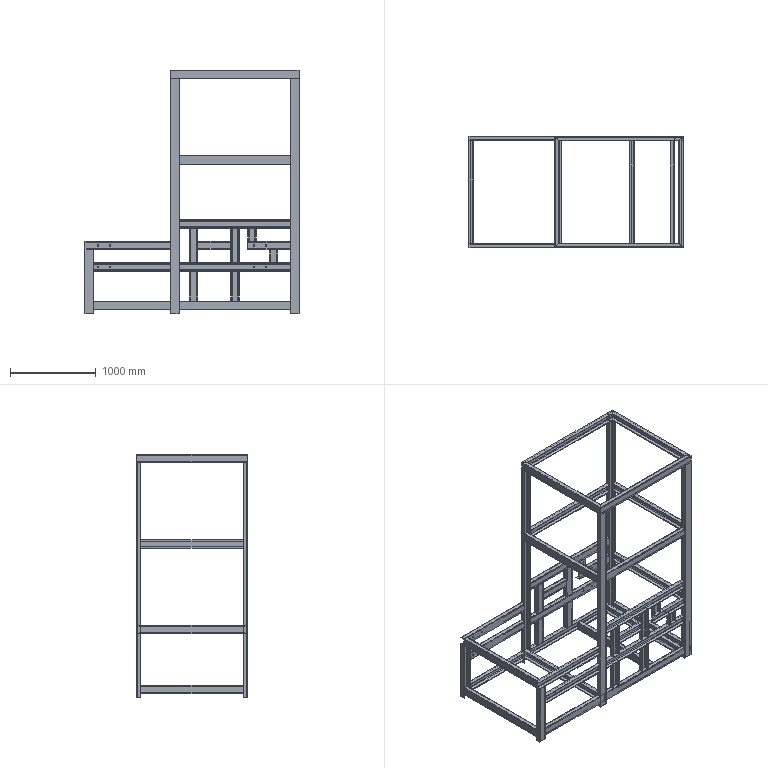Part | STEP file | Bracket 1XG(default_machined_) | 49 solids | 718 faces | box 2500 x 1300 x 2850 mm | volume 65972501 mm3 | plane 490 | cylinder 228 | commonest cylinder face diameters 9 x98 16 x98 17 x32